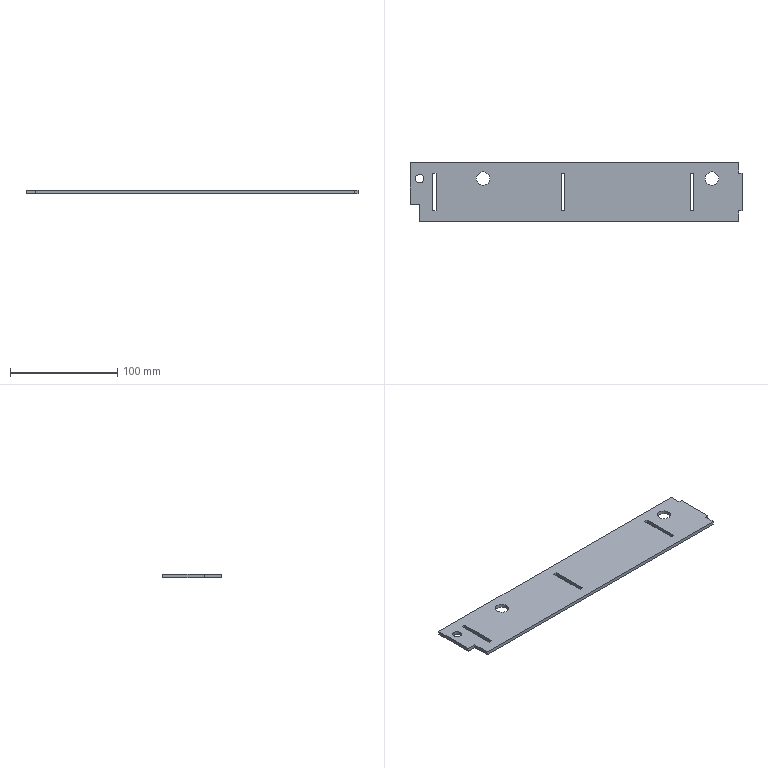Part | SolidWorks | features FlatPattern 1, SMBaseFlange 1, SheetMetal 1 | 1 solid | 30 faces | box 309 x 55 x 3.2 mm | volume 51735 mm3 | plane 24 | cylinder 6 | commonest cylinder face diameters 12.5 x4 8 x2
STEP:
#1=CARTESIAN_POINT('',(186.75,-15.,3.2));
#2=VERTEX_POINT('',#1);
#3=CARTESIAN_POINT('',(199.25,-15.,3.2));
#4=VERTEX_POINT('',#3);
#5=CARTESIAN_POINT('',(193.,-15.,3.2));
#6=DIRECTION('',(0.,0.,1.));
#7=DIRECTION('',(1.,0.,0.));
#8=AXIS2_PLACEMENT_3D('',#5,#6,#7);
#9=CIRCLE('',#8,6.25);
#10=EDGE_CURVE('',#2,#4,#9,.T.);
#11=ORIENTED_EDGE('',*,*,#10,.T.);
#12=CARTESIAN_POINT('',(199.25,-15.,0.));
#13=VERTEX_POINT('',#12);
#14=CARTESIAN_POINT('',(199.25,-15.,3.2));
#15=DIRECTION('',(0.,0.,-1.));
#16=VECTOR('',#15,1000.);
#17=LINE('',#14,#16);
#18=EDGE_CURVE('',#4,#13,#17,.T.);
#19=ORIENTED_EDGE('',*,*,#18,.T.);
#20=CARTESIAN_POINT('',(186.75,-15.,0.));
#21=VERTEX_POINT('',#20);
#22=CARTESIAN_POINT('',(193.,-15.,0.));
#23=DIRECTION('',(0.,0.,1.));
#24=DIRECTION('',(1.,0.,0.));
#25=AXIS2_PLACEMENT_3D('',#22,#23,#24);
#26=CIRCLE('',#25,6.25);
#27=EDGE_CURVE('',#21,#13,#26,.T.);
#28=ORIENTED_EDGE('',*,*,#27,.F.);
#29=CARTESIAN_POINT('',(186.75,-15.,3.2));
#30=DIRECTION('',(0.,0.,-1.));
#31=VECTOR('',#30,1000.);
#32=LINE('',#29,#31);
#33=EDGE_CURVE('',#2,#21,#32,.T.);
#34=ORIENTED_EDGE('',*,*,#33,.F.);
#35=EDGE_LOOP('',(#11,#19,#28,#34));
#36=FACE_OUTER_BOUND('',#35,.T.);
#37=CARTESIAN_POINT('',(193.,-15.,3.2));
#38=DIRECTION('',(0.,0.,-1.));
#39=DIRECTION('',(-1.,0.,0.));
#40=AXIS2_PLACEMENT_3D('',#37,#38,#39);
#41=CYLINDRICAL_SURFACE('',#40,6.25);
#42=ADVANCED_FACE('',(#36),#41,.F.);
#43=CARTESIAN_POINT('',(-26.25,-15.,3.2));
#44=VERTEX_POINT('',#43);
#45=CARTESIAN_POINT('',(-13.75,-15.,3.2));
#46=VERTEX_POINT('',#45);
#47=CARTESIAN_POINT('',(-20.,-15.,3.2));
#48=DIRECTION('',(0.,0.,1.));
#49=DIRECTION('',(1.,0.,0.));
#50=AXIS2_PLACEMENT_3D('',#47,#48,#49);
#51=CIRCLE('',#50,6.25);
#52=EDGE_CURVE('',#44,#46,#51,.T.);
#53=ORIENTED_EDGE('',*,*,#52,.T.);
#54=CARTESIAN_POINT('',(-13.75,-15.,0.));
#55=VERTEX_POINT('',#54);
#56=CARTESIAN_POINT('',(-13.75,-15.,3.2));
#57=DIRECTION('',(0.,0.,-1.));
#58=VECTOR('',#57,1000.);
#59=LINE('',#56,#58);
#60=EDGE_CURVE('',#46,#55,#59,.T.);
#61=ORIENTED_EDGE('',*,*,#60,.T.);
#62=CARTESIAN_POINT('',(-26.25,-15.,0.));
#63=VERTEX_POINT('',#62);
#64=CARTESIAN_POINT('',(-20.,-15.,0.));
#65=DIRECTION('',(0.,0.,1.));
#66=DIRECTION('',(1.,0.,0.));
#67=AXIS2_PLACEMENT_3D('',#64,#65,#66);
#68=CIRCLE('',#67,6.25);
#69=EDGE_CURVE('',#63,#55,#68,.T.);
#70=ORIENTED_EDGE('',*,*,#69,.F.);
#71=CARTESIAN_POINT('',(-26.25,-15.,3.2));
#72=DIRECTION('',(0.,0.,-1.));
#73=VECTOR('',#72,1000.);
#74=LINE('',#71,#73);
#75=EDGE_CURVE('',#44,#63,#74,.T.);
#76=ORIENTED_EDGE('',*,*,#75,.F.);
#77=EDGE_LOOP('',(#53,#61,#70,#76));
#78=FACE_OUTER_BOUND('',#77,.T.);
#79=CARTESIAN_POINT('',(-20.,-15.,3.2));
#80=DIRECTION('',(0.,0.,-1.));
#81=DIRECTION('',(-1.,0.,0.));
#82=AXIS2_PLACEMENT_3D('',#79,#80,#81);
#83=CYLINDRICAL_SURFACE('',#82,6.25);
#84=ADVANCED_FACE('',(#78),#83,.F.);
#85=CARTESIAN_POINT('',(-83.,-15.,3.2));
#86=VERTEX_POINT('',#85);
#87=CARTESIAN_POINT('',(-75.,-15.,3.2));
#88=VERTEX_POINT('',#87);
#89=CARTESIAN_POINT('',(-79.,-15.,3.2));
#90=DIRECTION('',(0.,0.,1.));
#91=DIRECTION('',(1.,0.,0.));
#92=AXIS2_PLACEMENT_3D('',#89,#90,#91);
#93=CIRCLE('',#92,4.);
#94=EDGE_CURVE('',#86,#88,#93,.T.);
#95=ORIENTED_EDGE('',*,*,#94,.T.);
#96=CARTESIAN_POINT('',(-75.,-15.,0.));
#97=VERTEX_POINT('',#96);
#98=CARTESIAN_POINT('',(-75.,-15.,3.2));
#99=DIRECTION('',(0.,0.,-1.));
#100=VECTOR('',#99,1000.);
#101=LINE('',#98,#100);
#102=EDGE_CURVE('',#88,#97,#101,.T.);
#103=ORIENTED_EDGE('',*,*,#102,.T.);
#104=CARTESIAN_POINT('',(-83.,-15.,0.));
#105=VERTEX_POINT('',#104);
#106=CARTESIAN_POINT('',(-79.,-15.,0.));
#107=DIRECTION('',(0.,0.,1.));
#108=DIRECTION('',(1.,0.,0.));
#109=AXIS2_PLACEMENT_3D('',#106,#107,#108);
#110=CIRCLE('',#109,4.);
#111=EDGE_CURVE('',#105,#97,#110,.T.);
#112=ORIENTED_EDGE('',*,*,#111,.F.);
#113=CARTESIAN_POINT('',(-83.,-15.,3.2));
#114=DIRECTION('',(0.,0.,-1.));
#115=VECTOR('',#114,1000.);
#116=LINE('',#113,#115);
#117=EDGE_CURVE('',#86,#105,#116,.T.);
#118=ORIENTED_EDGE('',*,*,#117,.F.);
#119=EDGE_LOOP('',(#95,#103,#112,#118));
#120=FACE_OUTER_BOUND('',#119,.T.);
#121=CARTESIAN_POINT('',(-79.,-15.,3.2));
#122=DIRECTION('',(0.,0.,-1.));
#123=DIRECTION('',(-1.,0.,0.));
#124=AXIS2_PLACEMENT_3D('',#121,#122,#123);
#125=CYLINDRICAL_SURFACE('',#124,4.);
#126=ADVANCED_FACE('',(#120),#125,.F.);
#127=ORIENTED_EDGE('',*,*,#52,.F.);
#128=CARTESIAN_POINT('',(-20.,-15.,3.2));
#129=DIRECTION('',(0.,0.,1.));
#130=DIRECTION('',(1.,0.,0.));
#131=AXIS2_PLACEMENT_3D('',#128,#129,#130);
#132=CIRCLE('',#131,6.25);
#133=EDGE_CURVE('',#46,#44,#132,.T.);
#134=ORIENTED_EDGE('',*,*,#133,.F.);
#135=EDGE_LOOP('',(#127,#134));
#136=FACE_BOUND('',#135,.T.);
#137=CARTESIAN_POINT('',(-67.,-45.,3.2));
#138=VERTEX_POINT('',#137);
#139=CARTESIAN_POINT('',(-63.8,-45.,3.2));
#140=VERTEX_POINT('',#139);
#141=CARTESIAN_POINT('',(-67.,-45.,3.2));
#142=DIRECTION('',(1.,0.,0.));
#143=VECTOR('',#142,1000.);
#144=LINE('',#141,#143);
#145=EDGE_CURVE('',#138,#140,#144,.T.);
#146=ORIENTED_EDGE('',*,*,#145,.F.);
#147=CARTESIAN_POINT('',(-67.,-10.,3.2));
#148=VERTEX_POINT('',#147);
#149=CARTESIAN_POINT('',(-67.,-45.,3.2));
#150=DIRECTION('',(0.,-1.,0.));
#151=VECTOR('',#150,1000.);
#152=LINE('',#149,#151);
#153=EDGE_CURVE('',#148,#138,#152,.T.);
#154=ORIENTED_EDGE('',*,*,#153,.F.);
#155=CARTESIAN_POINT('',(-63.8,-10.,3.2));
#156=VERTEX_POINT('',#155);
#157=CARTESIAN_POINT('',(-67.,-10.,3.2));
#158=DIRECTION('',(-1.,0.,0.));
#159=VECTOR('',#158,1000.);
#160=LINE('',#157,#159);
#161=EDGE_CURVE('',#156,#148,#160,.T.);
#162=ORIENTED_EDGE('',*,*,#161,.F.);
#163=CARTESIAN_POINT('',(-63.8,-45.,3.2));
#164=DIRECTION('',(0.,1.,0.));
#165=VECTOR('',#164,1000.);
#166=LINE('',#163,#165);
#167=EDGE_CURVE('',#140,#156,#166,.T.);
#168=ORIENTED_EDGE('',*,*,#167,.F.);
#169=EDGE_LOOP('',(#146,#154,#162,#168));
#170=FACE_BOUND('',#169,.T.);
#171=CARTESIAN_POINT('',(-88.,-39.,3.2));
#172=VERTEX_POINT('',#171);
#173=CARTESIAN_POINT('',(-79.5,-39.,3.2));
#174=VERTEX_POINT('',#173);
#175=CARTESIAN_POINT('',(-88.,-39.,3.2));
#176=DIRECTION('',(1.,0.,0.));
#177=VECTOR('',#176,1000.);
#178=LINE('',#175,#177);
#179=EDGE_CURVE('',#172,#174,#178,.T.);
#180=ORIENTED_EDGE('',*,*,#179,.T.);
#181=CARTESIAN_POINT('',(-79.5,-55.,3.2));
#182=VERTEX_POINT('',#181);
#183=CARTESIAN_POINT('',(-79.5,-55.,3.2));
#184=DIRECTION('',(0.,-1.,0.));
#185=VECTOR('',#184,1000.);
#186=LINE('',#183,#185);
#187=EDGE_CURVE('',#174,#182,#186,.T.);
#188=ORIENTED_EDGE('',*,*,#187,.T.);
#189=CARTESIAN_POINT('',(218.,-55.,3.2));
#190=VERTEX_POINT('',#189);
#191=CARTESIAN_POINT('',(218.,-55.,3.2));
#192=DIRECTION('',(1.,0.,0.));
#193=VECTOR('',#192,1000.);
#194=LINE('',#191,#193);
#195=EDGE_CURVE('',#182,#190,#194,.T.);
#196=ORIENTED_EDGE('',*,*,#195,.T.);
#197=CARTESIAN_POINT('',(218.,-45.,3.2));
#198=VERTEX_POINT('',#197);
#199=CARTESIAN_POINT('',(218.,-45.,3.2));
#200=DIRECTION('',(0.,1.,0.));
#201=VECTOR('',#200,1000.);
#202=LINE('',#199,#201);
#203=EDGE_CURVE('',#190,#198,#202,.T.);
#204=ORIENTED_EDGE('',*,*,#203,.T.);
#205=CARTESIAN_POINT('',(221.,-45.,3.2));
#206=VERTEX_POINT('',#205);
#207=CARTESIAN_POINT('',(221.,-45.,3.2));
#208=DIRECTION('',(1.,0.,0.));
#209=VECTOR('',#208,1000.);
#210=LINE('',#207,#209);
#211=EDGE_CURVE('',#198,#206,#210,.T.);
#212=ORIENTED_EDGE('',*,*,#211,.T.);
#213=CARTESIAN_POINT('',(221.,-10.,3.2));
#214=VERTEX_POINT('',#213);
#215=CARTESIAN_POINT('',(221.,-10.,3.2));
#216=DIRECTION('',(0.,1.,0.));
#217=VECTOR('',#216,1000.);
#218=LINE('',#215,#217);
#219=EDGE_CURVE('',#206,#214,#218,.T.);
#220=ORIENTED_EDGE('',*,*,#219,.T.);
#221=CARTESIAN_POINT('',(218.,-10.,3.2));
#222=VERTEX_POINT('',#221);
#223=CARTESIAN_POINT('',(218.,-10.,3.2));
#224=DIRECTION('',(-1.,0.,0.));
#225=VECTOR('',#224,1000.);
#226=LINE('',#223,#225);
#227=EDGE_CURVE('',#214,#222,#226,.T.);
#228=ORIENTED_EDGE('',*,*,#227,.T.);
#229=CARTESIAN_POINT('',(218.,0.,3.2));
#230=VERTEX_POINT('',#229);
#231=CARTESIAN_POINT('',(218.,0.,3.2));
#232=DIRECTION('',(0.,1.,0.));
#233=VECTOR('',#232,1000.);
#234=LINE('',#231,#233);
#235=EDGE_CURVE('',#222,#230,#234,.T.);
#236=ORIENTED_EDGE('',*,*,#235,.T.);
#237=CARTESIAN_POINT('',(-88.,0.,3.2));
#238=VERTEX_POINT('',#237);
#239=CARTESIAN_POINT('',(-88.,0.,3.2));
#240=DIRECTION('',(-1.,0.,0.));
#241=VECTOR('',#240,1000.);
#242=LINE('',#239,#241);
#243=EDGE_CURVE('',#230,#238,#242,.T.);
#244=ORIENTED_EDGE('',*,*,#243,.T.);
#245=CARTESIAN_POINT('',(-88.,0.,3.2));
#246=DIRECTION('',(0.,-1.,0.));
#247=VECTOR('',#246,1000.);
#248=LINE('',#245,#247);
#249=EDGE_CURVE('',#238,#172,#248,.T.);
#250=ORIENTED_EDGE('',*,*,#249,.T.);
#251=EDGE_LOOP('',(#180,#188,#196,#204,#212,#220,#228,#236,#244,#250));
#252=FACE_OUTER_BOUND('',#251,.T.);
#253=ORIENTED_EDGE('',*,*,#94,.F.);
#254=CARTESIAN_POINT('',(-79.,-15.,3.2));
#255=DIRECTION('',(0.,0.,1.));
#256=DIRECTION('',(1.,0.,0.));
#257=AXIS2_PLACEMENT_3D('',#254,#255,#256);
#258=CIRCLE('',#257,4.);
#259=EDGE_CURVE('',#88,#86,#258,.T.);
#260=ORIENTED_EDGE('',*,*,#259,.F.);
#261=EDGE_LOOP('',(#253,#260));
#262=FACE_BOUND('',#261,.T.);
#263=ORIENTED_EDGE('',*,*,#10,.F.);
#264=CARTESIAN_POINT('',(193.,-15.,3.2));
#265=DIRECTION('',(0.,0.,1.));
#266=DIRECTION('',(1.,0.,0.));
#267=AXIS2_PLACEMENT_3D('',#264,#265,#266);
#268=CIRCLE('',#267,6.25);
#269=EDGE_CURVE('',#4,#2,#268,.T.);
#270=ORIENTED_EDGE('',*,*,#269,.F.);
#271=EDGE_LOOP('',(#263,#270));
#272=FACE_BOUND('',#271,.T.);
#273=CARTESIAN_POINT('',(53.,-45.,3.2));
#274=VERTEX_POINT('',#273);
#275=CARTESIAN_POINT('',(56.2,-45.,3.2));
#276=VERTEX_POINT('',#275);
#277=CARTESIAN_POINT('',(53.,-45.,3.2));
#278=DIRECTION('',(1.,0.,0.));
#279=VECTOR('',#278,1000.);
#280=LINE('',#277,#279);
#281=EDGE_CURVE('',#274,#276,#280,.T.);
#282=ORIENTED_EDGE('',*,*,#281,.F.);
#283=CARTESIAN_POINT('',(53.,-10.,3.2));
#284=VERTEX_POINT('',#283);
#285=CARTESIAN_POINT('',(53.,-45.,3.2));
#286=DIRECTION('',(0.,-1.,0.));
#287=VECTOR('',#286,1000.);
#288=LINE('',#285,#287);
#289=EDGE_CURVE('',#284,#274,#288,.T.);
#290=ORIENTED_EDGE('',*,*,#289,.F.);
#291=CARTESIAN_POINT('',(56.2,-10.,3.2));
#292=VERTEX_POINT('',#291);
#293=CARTESIAN_POINT('',(53.,-10.,3.2));
#294=DIRECTION('',(-1.,0.,0.));
#295=VECTOR('',#294,1000.);
#296=LINE('',#293,#295);
#297=EDGE_CURVE('',#292,#284,#296,.T.);
#298=ORIENTED_EDGE('',*,*,#297,.F.);
#299=CARTESIAN_POINT('',(56.2,-45.,3.2));
#300=DIRECTION('',(0.,1.,0.));
#301=VECTOR('',#300,1000.);
#302=LINE('',#299,#301);
#303=EDGE_CURVE('',#276,#292,#302,.T.);
#304=ORIENTED_EDGE('',*,*,#303,.F.);
#305=EDGE_LOOP('',(#282,#290,#298,#304));
#306=FACE_BOUND('',#305,.T.);
#307=CARTESIAN_POINT('',(173.,-45.,3.2));
#308=VERTEX_POINT('',#307);
#309=CARTESIAN_POINT('',(176.2,-45.,3.2));
#310=VERTEX_POINT('',#309);
#311=CARTESIAN_POINT('',(173.,-45.,3.2));
#312=DIRECTION('',(1.,0.,0.));
#313=VECTOR('',#312,1000.);
#314=LINE('',#311,#313);
#315=EDGE_CURVE('',#308,#310,#314,.T.);
#316=ORIENTED_EDGE('',*,*,#315,.F.);
#317=CARTESIAN_POINT('',(173.,-10.,3.2));
#318=VERTEX_POINT('',#317);
#319=CARTESIAN_POINT('',(173.,-45.,3.2));
#320=DIRECTION('',(0.,-1.,0.));
#321=VECTOR('',#320,1000.);
#322=LINE('',#319,#321);
#323=EDGE_CURVE('',#318,#308,#322,.T.);
#324=ORIENTED_EDGE('',*,*,#323,.F.);
#325=CARTESIAN_POINT('',(176.2,-10.,3.2));
#326=VERTEX_POINT('',#325);
#327=CARTESIAN_POINT('',(173.,-10.,3.2));
#328=DIRECTION('',(-1.,0.,0.));
#329=VECTOR('',#328,1000.);
#330=LINE('',#327,#329);
#331=EDGE_CURVE('',#326,#318,#330,.T.);
#332=ORIENTED_EDGE('',*,*,#331,.F.);
#333=CARTESIAN_POINT('',(176.2,-45.,3.2));
#334=DIRECTION('',(0.,1.,0.));
#335=VECTOR('',#334,1000.);
#336=LINE('',#333,#335);
#337=EDGE_CURVE('',#310,#326,#336,.T.);
#338=ORIENTED_EDGE('',*,*,#337,.F.);
#339=EDGE_LOOP('',(#316,#324,#332,#338));
#340=FACE_BOUND('',#339,.T.);
#341=CARTESIAN_POINT('',(0.,0.,3.2));
#342=DIRECTION('',(0.,0.,1.));
#343=DIRECTION('',(1.,0.,0.));
#344=AXIS2_PLACEMENT_3D('',#341,#342,#343);
#345=PLANE('',#344);
#346=ADVANCED_FACE('',(#136,#170,#252,#262,#272,#306,#340),#345,.T.);
#347=CARTESIAN_POINT('',(53.,-10.,0.));
#348=VERTEX_POINT('',#347);
#349=CARTESIAN_POINT('',(53.,-45.,0.));
#350=VERTEX_POINT('',#349);
#351=CARTESIAN_POINT('',(53.,-45.,0.));
#352=DIRECTION('',(0.,-1.,0.));
#353=VECTOR('',#352,1000.);
#354=LINE('',#351,#353);
#355=EDGE_CURVE('',#348,#350,#354,.T.);
#356=ORIENTED_EDGE('',*,*,#355,.T.);
#357=CARTESIAN_POINT('',(56.2,-45.,0.));
#358=VERTEX_POINT('',#357);
#359=CARTESIAN_POINT('',(53.,-45.,0.));
#360=DIRECTION('',(1.,0.,0.));
#361=VECTOR('',#360,1000.);
#362=LINE('',#359,#361);
#363=EDGE_CURVE('',#350,#358,#362,.T.);
#364=ORIENTED_EDGE('',*,*,#363,.T.);
#365=CARTESIAN_POINT('',(56.2,-10.,0.));
#366=VERTEX_POINT('',#365);
#367=CARTESIAN_POINT('',(56.2,-45.,0.));
#368=DIRECTION('',(0.,1.,0.));
#369=VECTOR('',#368,1000.);
#370=LINE('',#367,#369);
#371=EDGE_CURVE('',#358,#366,#370,.T.);
#372=ORIENTED_EDGE('',*,*,#371,.T.);
#373=CARTESIAN_POINT('',(53.,-10.,0.));
#374=DIRECTION('',(-1.,0.,0.));
#375=VECTOR('',#374,1000.);
#376=LINE('',#373,#375);
#377=EDGE_CURVE('',#366,#348,#376,.T.);
#378=ORIENTED_EDGE('',*,*,#377,.T.);
#379=EDGE_LOOP('',(#356,#364,#372,#378));
#380=FACE_BOUND('',#379,.T.);
#381=CARTESIAN_POINT('',(-88.,-39.,0.));
#382=VERTEX_POINT('',#381);
#383=CARTESIAN_POINT('',(-79.5,-39.,0.));
#384=VERTEX_POINT('',#383);
#385=CARTESIAN_POINT('',(-88.,-39.,0.));
#386=DIRECTION('',(1.,0.,0.));
#387=VECTOR('',#386,1000.);
#388=LINE('',#385,#387);
#389=EDGE_CURVE('',#382,#384,#388,.T.);
#390=ORIENTED_EDGE('',*,*,#389,.F.);
#391=CARTESIAN_POINT('',(-88.,0.,0.));
#392=VERTEX_POINT('',#391);
#393=CARTESIAN_POINT('',(-88.,0.,0.));
#394=DIRECTION('',(0.,-1.,0.));
#395=VECTOR('',#394,1000.);
#396=LINE('',#393,#395);
#397=EDGE_CURVE('',#392,#382,#396,.T.);
#398=ORIENTED_EDGE('',*,*,#397,.F.);
#399=CARTESIAN_POINT('',(218.,0.,0.));
#400=VERTEX_POINT('',#399);
#401=CARTESIAN_POINT('',(-88.,0.,0.));
#402=DIRECTION('',(-1.,0.,0.));
#403=VECTOR('',#402,1000.);
#404=LINE('',#401,#403);
#405=EDGE_CURVE('',#400,#392,#404,.T.);
#406=ORIENTED_EDGE('',*,*,#405,.F.);
#407=CARTESIAN_POINT('',(218.,-10.,0.));
#408=VERTEX_POINT('',#407);
#409=CARTESIAN_POINT('',(218.,0.,0.));
#410=DIRECTION('',(0.,1.,0.));
#411=VECTOR('',#410,1000.);
#412=LINE('',#409,#411);
#413=EDGE_CURVE('',#408,#400,#412,.T.);
#414=ORIENTED_EDGE('',*,*,#413,.F.);
#415=CARTESIAN_POINT('',(221.,-10.,0.));
#416=VERTEX_POINT('',#415);
#417=CARTESIAN_POINT('',(218.,-10.,0.));
#418=DIRECTION('',(-1.,0.,0.));
#419=VECTOR('',#418,1000.);
#420=LINE('',#417,#419);
#421=EDGE_CURVE('',#416,#408,#420,.T.);
#422=ORIENTED_EDGE('',*,*,#421,.F.);
#423=CARTESIAN_POINT('',(221.,-45.,0.));
#424=VERTEX_POINT('',#423);
#425=CARTESIAN_POINT('',(221.,-10.,0.));
#426=DIRECTION('',(0.,1.,0.));
#427=VECTOR('',#426,1000.);
#428=LINE('',#425,#427);
#429=EDGE_CURVE('',#424,#416,#428,.T.);
#430=ORIENTED_EDGE('',*,*,#429,.F.);
#431=CARTESIAN_POINT('',(218.,-45.,0.));
#432=VERTEX_POINT('',#431);
#433=CARTESIAN_POINT('',(221.,-45.,0.));
#434=DIRECTION('',(1.,0.,0.));
#435=VECTOR('',#434,1000.);
#436=LINE('',#433,#435);
#437=EDGE_CURVE('',#432,#424,#436,.T.);
#438=ORIENTED_EDGE('',*,*,#437,.F.);
#439=CARTESIAN_POINT('',(218.,-55.,0.));
#440=VERTEX_POINT('',#439);
#441=CARTESIAN_POINT('',(218.,-45.,0.));
#442=DIRECTION('',(0.,1.,0.));
#443=VECTOR('',#442,1000.);
#444=LINE('',#441,#443);
#445=EDGE_CURVE('',#440,#432,#444,.T.);
#446=ORIENTED_EDGE('',*,*,#445,.F.);
#447=CARTESIAN_POINT('',(-79.5,-55.,0.));
#448=VERTEX_POINT('',#447);
#449=CARTESIAN_POINT('',(218.,-55.,0.));
#450=DIRECTION('',(1.,0.,0.));
#451=VECTOR('',#450,1000.);
#452=LINE('',#449,#451);
#453=EDGE_CURVE('',#448,#440,#452,.T.);
#454=ORIENTED_EDGE('',*,*,#453,.F.);
#455=CARTESIAN_POINT('',(-79.5,-55.,0.));
#456=DIRECTION('',(0.,-1.,0.));
#457=VECTOR('',#456,1000.);
#458=LINE('',#455,#457);
#459=EDGE_CURVE('',#384,#448,#458,.T.);
#460=ORIENTED_EDGE('',*,*,#459,.F.);
#461=EDGE_LOOP('',(#390,#398,#406,#414,#422,#430,#438,#446,#454,#460));
#462=FACE_OUTER_BOUND('',#461,.T.);
#463=CARTESIAN_POINT('',(-67.,-10.,0.));
#464=VERTEX_POINT('',#463);
#465=CARTESIAN_POINT('',(-67.,-45.,0.));
#466=VERTEX_POINT('',#465);
#467=CARTESIAN_POINT('',(-67.,-45.,0.));
#468=DIRECTION('',(0.,-1.,0.));
#469=VECTOR('',#468,1000.);
#470=LINE('',#467,#469);
#471=EDGE_CURVE('',#464,#466,#470,.T.);
#472=ORIENTED_EDGE('',*,*,#471,.T.);
#473=CARTESIAN_POINT('',(-63.8,-45.,0.));
#474=VERTEX_POINT('',#473);
#475=CARTESIAN_POINT('',(-67.,-45.,0.));
#476=DIRECTION('',(1.,0.,0.));
#477=VECTOR('',#476,1000.);
#478=LINE('',#475,#477);
#479=EDGE_CURVE('',#466,#474,#478,.T.);
#480=ORIENTED_EDGE('',*,*,#479,.T.);
#481=CARTESIAN_POINT('',(-63.8,-10.,0.));
#482=VERTEX_POINT('',#481);
#483=CARTESIAN_POINT('',(-63.8,-45.,0.));
#484=DIRECTION('',(0.,1.,0.));
#485=VECTOR('',#484,1000.);
#486=LINE('',#483,#485);
#487=EDGE_CURVE('',#474,#482,#486,.T.);
#488=ORIENTED_EDGE('',*,*,#487,.T.);
#489=CARTESIAN_POINT('',(-67.,-10.,0.));
#490=DIRECTION('',(-1.,0.,0.));
#491=VECTOR('',#490,1000.);
#492=LINE('',#489,#491);
#493=EDGE_CURVE('',#482,#464,#492,.T.);
#494=ORIENTED_EDGE('',*,*,#493,.T.);
#495=EDGE_LOOP('',(#472,#480,#488,#494));
#496=FACE_BOUND('',#495,.T.);
#497=ORIENTED_EDGE('',*,*,#111,.T.);
#498=CARTESIAN_POINT('',(-79.,-15.,0.));
#499=DIRECTION('',(0.,0.,1.));
#500=DIRECTION('',(1.,0.,0.));
#501=AXIS2_PLACEMENT_3D('',#498,#499,#500);
#502=CIRCLE('',#501,4.);
#503=EDGE_CURVE('',#97,#105,#502,.T.);
#504=ORIENTED_EDGE('',*,*,#503,.T.);
#505=EDGE_LOOP('',(#497,#504));
#506=FACE_BOUND('',#505,.T.);
#507=ORIENTED_EDGE('',*,*,#69,.T.);
#508=CARTESIAN_POINT('',(-20.,-15.,0.));
#509=DIRECTION('',(0.,0.,1.));
#510=DIRECTION('',(1.,0.,0.));
#511=AXIS2_PLACEMENT_3D('',#508,#509,#510);
#512=CIRCLE('',#511,6.25);
#513=EDGE_CURVE('',#55,#63,#512,.T.);
#514=ORIENTED_EDGE('',*,*,#513,.T.);
#515=EDGE_LOOP('',(#507,#514));
#516=FACE_BOUND('',#515,.T.);
#517=ORIENTED_EDGE('',*,*,#27,.T.);
#518=CARTESIAN_POINT('',(193.,-15.,0.));
#519=DIRECTION('',(0.,0.,1.));
#520=DIRECTION('',(1.,0.,0.));
#521=AXIS2_PLACEMENT_3D('',#518,#519,#520);
#522=CIRCLE('',#521,6.25);
#523=EDGE_CURVE('',#13,#21,#522,.T.);
#524=ORIENTED_EDGE('',*,*,#523,.T.);
#525=EDGE_LOOP('',(#517,#524));
#526=FACE_BOUND('',#525,.T.);
#527=CARTESIAN_POINT('',(173.,-10.,0.));
#528=VERTEX_POINT('',#527);
#529=CARTESIAN_POINT('',(173.,-45.,0.));
#530=VERTEX_POINT('',#529);
#531=CARTESIAN_POINT('',(173.,-45.,0.));
#532=DIRECTION('',(0.,-1.,0.));
#533=VECTOR('',#532,1000.);
#534=LINE('',#531,#533);
#535=EDGE_CURVE('',#528,#530,#534,.T.);
#536=ORIENTED_EDGE('',*,*,#535,.T.);
#537=CARTESIAN_POINT('',(176.2,-45.,0.));
#538=VERTEX_POINT('',#537);
#539=CARTESIAN_POINT('',(173.,-45.,0.));
#540=DIRECTION('',(1.,0.,0.));
#541=VECTOR('',#540,1000.);
#542=LINE('',#539,#541);
#543=EDGE_CURVE('',#530,#538,#542,.T.);
#544=ORIENTED_EDGE('',*,*,#543,.T.);
#545=CARTESIAN_POINT('',(176.2,-10.,0.));
#546=VERTEX_POINT('',#545);
#547=CARTESIAN_POINT('',(176.2,-45.,0.));
#548=DIRECTION('',(0.,1.,0.));
#549=VECTOR('',#548,1000.);
#550=LINE('',#547,#549);
#551=EDGE_CURVE('',#538,#546,#550,.T.);
#552=ORIENTED_EDGE('',*,*,#551,.T.);
#553=CARTESIAN_POINT('',(173.,-10.,0.));
#554=DIRECTION('',(-1.,0.,0.));
#555=VECTOR('',#554,1000.);
#556=LINE('',#553,#555);
#557=EDGE_CURVE('',#546,#528,#556,.T.);
#558=ORIENTED_EDGE('',*,*,#557,.T.);
#559=EDGE_LOOP('',(#536,#544,#552,#558));
#560=FACE_BOUND('',#559,.T.);
#561=CARTESIAN_POINT('',(0.,0.,0.));
#562=DIRECTION('',(0.,0.,1.));
#563=DIRECTION('',(1.,0.,0.));
#564=AXIS2_PLACEMENT_3D('',#561,#562,#563);
#565=PLANE('',#564);
#566=ADVANCED_FACE('',(#380,#462,#496,#506,#516,#526,#560),#565,.F.);
#567=ORIENTED_EDGE('',*,*,#389,.T.);
#568=CARTESIAN_POINT('',(-79.5,-39.,3.2));
#569=DIRECTION('',(0.,0.,-1.));
#570=VECTOR('',#569,1000.);
#571=LINE('',#568,#570);
#572=EDGE_CURVE('',#174,#384,#571,.T.);
#573=ORIENTED_EDGE('',*,*,#572,.F.);
#574=ORIENTED_EDGE('',*,*,#179,.F.);
#575=CARTESIAN_POINT('',(-88.,-39.,3.2));
#576=DIRECTION('',(0.,0.,-1.));
#577=VECTOR('',#576,1000.);
#578=LINE('',#575,#577);
#579=EDGE_CURVE('',#172,#382,#578,.T.);
#580=ORIENTED_EDGE('',*,*,#579,.T.);
#581=EDGE_LOOP('',(#567,#573,#574,#580));
#582=FACE_OUTER_BOUND('',#581,.T.);
#583=CARTESIAN_POINT('',(-88.,-39.,3.2));
#584=DIRECTION('',(0.,1.,0.));
#585=DIRECTION('',(0.,0.,1.));
#586=AXIS2_PLACEMENT_3D('',#583,#584,#585);
#587=PLANE('',#586);
#588=ADVANCED_FACE('',(#582),#587,.F.);
#589=ORIENTED_EDGE('',*,*,#459,.T.);
#590=CARTESIAN_POINT('',(-79.5,-55.,3.2));
#591=DIRECTION('',(0.,0.,-1.));
#592=VECTOR('',#591,1000.);
#593=LINE('',#590,#592);
#594=EDGE_CURVE('',#182,#448,#593,.T.);
#595=ORIENTED_EDGE('',*,*,#594,.F.);
#596=ORIENTED_EDGE('',*,*,#187,.F.);
#597=ORIENTED_EDGE('',*,*,#572,.T.);
#598=EDGE_LOOP('',(#589,#595,#596,#597));
#599=FACE_OUTER_BOUND('',#598,.T.);
#600=CARTESIAN_POINT('',(-79.5,-55.,3.2));
#601=DIRECTION('',(1.,0.,0.));
#602=DIRECTION('',(0.,0.,-1.));
#603=AXIS2_PLACEMENT_3D('',#600,#601,#602);
#604=PLANE('',#603);
#605=ADVANCED_FACE('',(#599),#604,.F.);
#606=ORIENTED_EDGE('',*,*,#453,.T.);
#607=CARTESIAN_POINT('',(218.,-55.,3.2));
#608=DIRECTION('',(0.,0.,-1.));
#609=VECTOR('',#608,1000.);
#610=LINE('',#607,#609);
#611=EDGE_CURVE('',#190,#440,#610,.T.);
#612=ORIENTED_EDGE('',*,*,#611,.F.);
#613=ORIENTED_EDGE('',*,*,#195,.F.);
#614=ORIENTED_EDGE('',*,*,#594,.T.);
#615=EDGE_LOOP('',(#606,#612,#613,#614));
#616=FACE_OUTER_BOUND('',#615,.T.);
#617=CARTESIAN_POINT('',(218.,-55.,3.2));
#618=DIRECTION('',(0.,1.,0.));
#619=DIRECTION('',(-1.,0.,0.));
#620=AXIS2_PLACEMENT_3D('',#617,#618,#619);
#621=PLANE('',#620);
#622=ADVANCED_FACE('',(#616),#621,.F.);
#623=ORIENTED_EDGE('',*,*,#445,.T.);
#624=CARTESIAN_POINT('',(218.,-45.,3.2));
#625=DIRECTION('',(0.,0.,-1.));
#626=VECTOR('',#625,1000.);
#627=LINE('',#624,#626);
#628=EDGE_CURVE('',#198,#432,#627,.T.);
#629=ORIENTED_EDGE('',*,*,#628,.F.);
#630=ORIENTED_EDGE('',*,*,#203,.F.);
#631=ORIENTED_EDGE('',*,*,#611,.T.);
#632=EDGE_LOOP('',(#623,#629,#630,#631));
#633=FACE_OUTER_BOUND('',#632,.T.);
#634=CARTESIAN_POINT('',(218.,-45.,3.2));
#635=DIRECTION('',(-1.,0.,0.));
#636=DIRECTION('',(0.,0.,1.));
#637=AXIS2_PLACEMENT_3D('',#634,#635,#636);
#638=PLANE('',#637);
#639=ADVANCED_FACE('',(#633),#638,.F.);
#640=ORIENTED_EDGE('',*,*,#437,.T.);
#641=CARTESIAN_POINT('',(221.,-45.,3.2));
#642=DIRECTION('',(0.,0.,-1.));
#643=VECTOR('',#642,1000.);
#644=LINE('',#641,#643);
#645=EDGE_CURVE('',#206,#424,#644,.T.);
#646=ORIENTED_EDGE('',*,*,#645,.F.);
#647=ORIENTED_EDGE('',*,*,#211,.F.);
#648=ORIENTED_EDGE('',*,*,#628,.T.);
#649=EDGE_LOOP('',(#640,#646,#647,#648));
#650=FACE_OUTER_BOUND('',#649,.T.);
#651=CARTESIAN_POINT('',(221.,-45.,3.2));
#652=DIRECTION('',(0.,1.,0.));
#653=DIRECTION('',(0.,0.,1.));
#654=AXIS2_PLACEMENT_3D('',#651,#652,#653);
#655=PLANE('',#654);
#656=ADVANCED_FACE('',(#650),#655,.F.);
#657=ORIENTED_EDGE('',*,*,#429,.T.);
#658=CARTESIAN_POINT('',(221.,-10.,3.2));
#659=DIRECTION('',(0.,0.,-1.));
#660=VECTOR('',#659,1000.);
#661=LINE('',#658,#660);
#662=EDGE_CURVE('',#214,#416,#661,.T.);
#663=ORIENTED_EDGE('',*,*,#662,.F.);
#664=ORIENTED_EDGE('',*,*,#219,.F.);
#665=ORIENTED_EDGE('',*,*,#645,.T.);
#666=EDGE_LOOP('',(#657,#663,#664,#665));
#667=FACE_OUTER_BOUND('',#666,.T.);
#668=CARTESIAN_POINT('',(221.,-10.,3.2));
#669=DIRECTION('',(-1.,0.,0.));
#670=DIRECTION('',(0.,0.,1.));
#671=AXIS2_PLACEMENT_3D('',#668,#669,#670);
#672=PLANE('',#671);
#673=ADVANCED_FACE('',(#667),#672,.F.);
#674=ORIENTED_EDGE('',*,*,#421,.T.);
#675=CARTESIAN_POINT('',(218.,-10.,3.2));
#676=DIRECTION('',(0.,0.,-1.));
#677=VECTOR('',#676,1000.);
#678=LINE('',#675,#677);
#679=EDGE_CURVE('',#222,#408,#678,.T.);
#680=ORIENTED_EDGE('',*,*,#679,.F.);
#681=ORIENTED_EDGE('',*,*,#227,.F.);
#682=ORIENTED_EDGE('',*,*,#662,.T.);
#683=EDGE_LOOP('',(#674,#680,#681,#682));
#684=FACE_OUTER_BOUND('',#683,.T.);
#685=CARTESIAN_POINT('',(218.,-10.,3.2));
#686=DIRECTION('',(0.,-1.,0.));
#687=DIRECTION('',(0.,0.,-1.));
#688=AXIS2_PLACEMENT_3D('',#685,#686,#687);
#689=PLANE('',#688);
#690=ADVANCED_FACE('',(#684),#689,.F.);
#691=ORIENTED_EDGE('',*,*,#413,.T.);
#692=CARTESIAN_POINT('',(218.,0.,3.2));
#693=DIRECTION('',(0.,0.,-1.));
#694=VECTOR('',#693,1000.);
#695=LINE('',#692,#694);
#696=EDGE_CURVE('',#230,#400,#695,.T.);
#697=ORIENTED_EDGE('',*,*,#696,.F.);
#698=ORIENTED_EDGE('',*,*,#235,.F.);
#699=ORIENTED_EDGE('',*,*,#679,.T.);
#700=EDGE_LOOP('',(#691,#697,#698,#699));
#701=FACE_OUTER_BOUND('',#700,.T.);
#702=CARTESIAN_POINT('',(218.,0.,3.2));
#703=DIRECTION('',(-1.,0.,0.));
#704=DIRECTION('',(0.,0.,1.));
#705=AXIS2_PLACEMENT_3D('',#702,#703,#704);
#706=PLANE('',#705);
#707=ADVANCED_FACE('',(#701),#706,.F.);
#708=ORIENTED_EDGE('',*,*,#405,.T.);
#709=CARTESIAN_POINT('',(-88.,0.,3.2));
#710=DIRECTION('',(0.,0.,-1.));
#711=VECTOR('',#710,1000.);
#712=LINE('',#709,#711);
#713=EDGE_CURVE('',#238,#392,#712,.T.);
#714=ORIENTED_EDGE('',*,*,#713,.F.);
#715=ORIENTED_EDGE('',*,*,#243,.F.);
#716=ORIENTED_EDGE('',*,*,#696,.T.);
#717=EDGE_LOOP('',(#708,#714,#715,#716));
#718=FACE_OUTER_BOUND('',#717,.T.);
#719=CARTESIAN_POINT('',(-88.,0.,3.2));
#720=DIRECTION('',(0.,-1.,0.));
#721=DIRECTION('',(1.,0.,0.));
#722=AXIS2_PLACEMENT_3D('',#719,#720,#721);
#723=PLANE('',#722);
#724=ADVANCED_FACE('',(#718),#723,.F.);
#725=ORIENTED_EDGE('',*,*,#397,.T.);
#726=ORIENTED_EDGE('',*,*,#579,.F.);
#727=ORIENTED_EDGE('',*,*,#249,.F.);
#728=ORIENTED_EDGE('',*,*,#713,.T.);
#729=EDGE_LOOP('',(#725,#726,#727,#728));
#730=FACE_OUTER_BOUND('',#729,.T.);
#731=CARTESIAN_POINT('',(-88.,0.,3.2));
#732=DIRECTION('',(1.,0.,0.));
#733=DIRECTION('',(0.,1.,0.));
#734=AXIS2_PLACEMENT_3D('',#731,#732,#733);
#735=PLANE('',#734);
#736=ADVANCED_FACE('',(#730),#735,.F.);
#737=ORIENTED_EDGE('',*,*,#471,.F.);
#738=CARTESIAN_POINT('',(-67.,-10.,3.2));
#739=DIRECTION('',(0.,0.,-1.));
#740=VECTOR('',#739,1000.);
#741=LINE('',#738,#740);
#742=EDGE_CURVE('',#148,#464,#741,.T.);
#743=ORIENTED_EDGE('',*,*,#742,.F.);
#744=ORIENTED_EDGE('',*,*,#153,.T.);
#745=CARTESIAN_POINT('',(-67.,-45.,3.2));
#746=DIRECTION('',(0.,0.,-1.));
#747=VECTOR('',#746,1000.);
#748=LINE('',#745,#747);
#749=EDGE_CURVE('',#138,#466,#748,.T.);
#750=ORIENTED_EDGE('',*,*,#749,.T.);
#751=EDGE_LOOP('',(#737,#743,#744,#750));
#752=FACE_OUTER_BOUND('',#751,.T.);
#753=CARTESIAN_POINT('',(-67.,-45.,3.2));
#754=DIRECTION('',(1.,0.,0.));
#755=DIRECTION('',(0.,0.,-1.));
#756=AXIS2_PLACEMENT_3D('',#753,#754,#755);
#757=PLANE('',#756);
#758=ADVANCED_FACE('',(#752),#757,.T.);
#759=ORIENTED_EDGE('',*,*,#479,.F.);
#760=ORIENTED_EDGE('',*,*,#749,.F.);
#761=ORIENTED_EDGE('',*,*,#145,.T.);
#762=CARTESIAN_POINT('',(-63.8,-45.,3.2));
#763=DIRECTION('',(0.,0.,-1.));
#764=VECTOR('',#763,1000.);
#765=LINE('',#762,#764);
#766=EDGE_CURVE('',#140,#474,#765,.T.);
#767=ORIENTED_EDGE('',*,*,#766,.T.);
#768=EDGE_LOOP('',(#759,#760,#761,#767));
#769=FACE_OUTER_BOUND('',#768,.T.);
#770=CARTESIAN_POINT('',(-67.,-45.,3.2));
#771=DIRECTION('',(0.,1.,0.));
#772=DIRECTION('',(0.,0.,1.));
#773=AXIS2_PLACEMENT_3D('',#770,#771,#772);
#774=PLANE('',#773);
#775=ADVANCED_FACE('',(#769),#774,.T.);
#776=ORIENTED_EDGE('',*,*,#487,.F.);
#777=ORIENTED_EDGE('',*,*,#766,.F.);
#778=ORIENTED_EDGE('',*,*,#167,.T.);
#779=CARTESIAN_POINT('',(-63.8,-10.,3.2));
#780=DIRECTION('',(0.,0.,-1.));
#781=VECTOR('',#780,1000.);
#782=LINE('',#779,#781);
#783=EDGE_CURVE('',#156,#482,#782,.T.);
#784=ORIENTED_EDGE('',*,*,#783,.T.);
#785=EDGE_LOOP('',(#776,#777,#778,#784));
#786=FACE_OUTER_BOUND('',#785,.T.);
#787=CARTESIAN_POINT('',(-63.8,-45.,3.2));
#788=DIRECTION('',(-1.,0.,0.));
#789=DIRECTION('',(0.,0.,1.));
#790=AXIS2_PLACEMENT_3D('',#787,#788,#789);
#791=PLANE('',#790);
#792=ADVANCED_FACE('',(#786),#791,.T.);
#793=ORIENTED_EDGE('',*,*,#493,.F.);
#794=ORIENTED_EDGE('',*,*,#783,.F.);
#795=ORIENTED_EDGE('',*,*,#161,.T.);
#796=ORIENTED_EDGE('',*,*,#742,.T.);
#797=EDGE_LOOP('',(#793,#794,#795,#796));
#798=FACE_OUTER_BOUND('',#797,.T.);
#799=CARTESIAN_POINT('',(-67.,-10.,3.2));
#800=DIRECTION('',(0.,-1.,0.));
#801=DIRECTION('',(0.,0.,-1.));
#802=AXIS2_PLACEMENT_3D('',#799,#800,#801);
#803=PLANE('',#802);
#804=ADVANCED_FACE('',(#798),#803,.T.);
#805=ORIENTED_EDGE('',*,*,#102,.F.);
#806=ORIENTED_EDGE('',*,*,#259,.T.);
#807=ORIENTED_EDGE('',*,*,#117,.T.);
#808=ORIENTED_EDGE('',*,*,#503,.F.);
#809=EDGE_LOOP('',(#805,#806,#807,#808));
#810=FACE_OUTER_BOUND('',#809,.T.);
#811=CARTESIAN_POINT('',(-79.,-15.,3.2));
#812=DIRECTION('',(0.,0.,-1.));
#813=DIRECTION('',(-1.,0.,0.));
#814=AXIS2_PLACEMENT_3D('',#811,#812,#813);
#815=CYLINDRICAL_SURFACE('',#814,4.);
#816=ADVANCED_FACE('',(#810),#815,.F.);
#817=ORIENTED_EDGE('',*,*,#60,.F.);
#818=ORIENTED_EDGE('',*,*,#133,.T.);
#819=ORIENTED_EDGE('',*,*,#75,.T.);
#820=ORIENTED_EDGE('',*,*,#513,.F.);
#821=EDGE_LOOP('',(#817,#818,#819,#820));
#822=FACE_OUTER_BOUND('',#821,.T.);
#823=CARTESIAN_POINT('',(-20.,-15.,3.2));
#824=DIRECTION('',(0.,0.,-1.));
#825=DIRECTION('',(-1.,0.,0.));
#826=AXIS2_PLACEMENT_3D('',#823,#824,#825);
#827=CYLINDRICAL_SURFACE('',#826,6.25);
#828=ADVANCED_FACE('',(#822),#827,.F.);
#829=ORIENTED_EDGE('',*,*,#18,.F.);
#830=ORIENTED_EDGE('',*,*,#269,.T.);
#831=ORIENTED_EDGE('',*,*,#33,.T.);
#832=ORIENTED_EDGE('',*,*,#523,.F.);
#833=EDGE_LOOP('',(#829,#830,#831,#832));
#834=FACE_OUTER_BOUND('',#833,.T.);
#835=CARTESIAN_POINT('',(193.,-15.,3.2));
#836=DIRECTION('',(0.,0.,-1.));
#837=DIRECTION('',(-1.,0.,0.));
#838=AXIS2_PLACEMENT_3D('',#835,#836,#837);
#839=CYLINDRICAL_SURFACE('',#838,6.25);
#840=ADVANCED_FACE('',(#834),#839,.F.);
#841=ORIENTED_EDGE('',*,*,#355,.F.);
#842=CARTESIAN_POINT('',(53.,-10.,3.2));
#843=DIRECTION('',(0.,0.,-1.));
#844=VECTOR('',#843,1000.);
#845=LINE('',#842,#844);
#846=EDGE_CURVE('',#284,#348,#845,.T.);
#847=ORIENTED_EDGE('',*,*,#846,.F.);
#848=ORIENTED_EDGE('',*,*,#289,.T.);
#849=CARTESIAN_POINT('',(53.,-45.,3.2));
#850=DIRECTION('',(0.,0.,-1.));
#851=VECTOR('',#850,1000.);
#852=LINE('',#849,#851);
#853=EDGE_CURVE('',#274,#350,#852,.T.);
#854=ORIENTED_EDGE('',*,*,#853,.T.);
#855=EDGE_LOOP('',(#841,#847,#848,#854));
#856=FACE_OUTER_BOUND('',#855,.T.);
#857=CARTESIAN_POINT('',(53.,-45.,3.2));
#858=DIRECTION('',(1.,0.,0.));
#859=DIRECTION('',(0.,0.,-1.));
#860=AXIS2_PLACEMENT_3D('',#857,#858,#859);
#861=PLANE('',#860);
#862=ADVANCED_FACE('',(#856),#861,.T.);
#863=ORIENTED_EDGE('',*,*,#363,.F.);
#864=ORIENTED_EDGE('',*,*,#853,.F.);
#865=ORIENTED_EDGE('',*,*,#281,.T.);
#866=CARTESIAN_POINT('',(56.2,-45.,3.2));
#867=DIRECTION('',(0.,0.,-1.));
#868=VECTOR('',#867,1000.);
#869=LINE('',#866,#868);
#870=EDGE_CURVE('',#276,#358,#869,.T.);
#871=ORIENTED_EDGE('',*,*,#870,.T.);
#872=EDGE_LOOP('',(#863,#864,#865,#871));
#873=FACE_OUTER_BOUND('',#872,.T.);
#874=CARTESIAN_POINT('',(53.,-45.,3.2));
#875=DIRECTION('',(0.,1.,0.));
#876=DIRECTION('',(0.,0.,1.));
#877=AXIS2_PLACEMENT_3D('',#874,#875,#876);
#878=PLANE('',#877);
#879=ADVANCED_FACE('',(#873),#878,.T.);
#880=ORIENTED_EDGE('',*,*,#371,.F.);
#881=ORIENTED_EDGE('',*,*,#870,.F.);
#882=ORIENTED_EDGE('',*,*,#303,.T.);
#883=CARTESIAN_POINT('',(56.2,-10.,3.2));
#884=DIRECTION('',(0.,0.,-1.));
#885=VECTOR('',#884,1000.);
#886=LINE('',#883,#885);
#887=EDGE_CURVE('',#292,#366,#886,.T.);
#888=ORIENTED_EDGE('',*,*,#887,.T.);
#889=EDGE_LOOP('',(#880,#881,#882,#888));
#890=FACE_OUTER_BOUND('',#889,.T.);
#891=CARTESIAN_POINT('',(56.2,-45.,3.2));
#892=DIRECTION('',(-1.,0.,0.));
#893=DIRECTION('',(0.,0.,1.));
#894=AXIS2_PLACEMENT_3D('',#891,#892,#893);
#895=PLANE('',#894);
#896=ADVANCED_FACE('',(#890),#895,.T.);
#897=ORIENTED_EDGE('',*,*,#377,.F.);
#898=ORIENTED_EDGE('',*,*,#887,.F.);
#899=ORIENTED_EDGE('',*,*,#297,.T.);
#900=ORIENTED_EDGE('',*,*,#846,.T.);
#901=EDGE_LOOP('',(#897,#898,#899,#900));
#902=FACE_OUTER_BOUND('',#901,.T.);
#903=CARTESIAN_POINT('',(53.,-10.,3.2));
#904=DIRECTION('',(0.,-1.,0.));
#905=DIRECTION('',(0.,0.,-1.));
#906=AXIS2_PLACEMENT_3D('',#903,#904,#905);
#907=PLANE('',#906);
#908=ADVANCED_FACE('',(#902),#907,.T.);
#909=ORIENTED_EDGE('',*,*,#535,.F.);
#910=CARTESIAN_POINT('',(173.,-10.,3.2));
#911=DIRECTION('',(0.,0.,-1.));
#912=VECTOR('',#911,1000.);
#913=LINE('',#910,#912);
#914=EDGE_CURVE('',#318,#528,#913,.T.);
#915=ORIENTED_EDGE('',*,*,#914,.F.);
#916=ORIENTED_EDGE('',*,*,#323,.T.);
#917=CARTESIAN_POINT('',(173.,-45.,3.2));
#918=DIRECTION('',(0.,0.,-1.));
#919=VECTOR('',#918,1000.);
#920=LINE('',#917,#919);
#921=EDGE_CURVE('',#308,#530,#920,.T.);
#922=ORIENTED_EDGE('',*,*,#921,.T.);
#923=EDGE_LOOP('',(#909,#915,#916,#922));
#924=FACE_OUTER_BOUND('',#923,.T.);
#925=CARTESIAN_POINT('',(173.,-45.,3.2));
#926=DIRECTION('',(1.,0.,0.));
#927=DIRECTION('',(0.,0.,-1.));
#928=AXIS2_PLACEMENT_3D('',#925,#926,#927);
#929=PLANE('',#928);
#930=ADVANCED_FACE('',(#924),#929,.T.);
#931=ORIENTED_EDGE('',*,*,#543,.F.);
#932=ORIENTED_EDGE('',*,*,#921,.F.);
#933=ORIENTED_EDGE('',*,*,#315,.T.);
#934=CARTESIAN_POINT('',(176.2,-45.,3.2));
#935=DIRECTION('',(0.,0.,-1.));
#936=VECTOR('',#935,1000.);
#937=LINE('',#934,#936);
#938=EDGE_CURVE('',#310,#538,#937,.T.);
#939=ORIENTED_EDGE('',*,*,#938,.T.);
#940=EDGE_LOOP('',(#931,#932,#933,#939));
#941=FACE_OUTER_BOUND('',#940,.T.);
#942=CARTESIAN_POINT('',(173.,-45.,3.2));
#943=DIRECTION('',(0.,1.,0.));
#944=DIRECTION('',(0.,0.,1.));
#945=AXIS2_PLACEMENT_3D('',#942,#943,#944);
#946=PLANE('',#945);
#947=ADVANCED_FACE('',(#941),#946,.T.);
#948=ORIENTED_EDGE('',*,*,#551,.F.);
#949=ORIENTED_EDGE('',*,*,#938,.F.);
#950=ORIENTED_EDGE('',*,*,#337,.T.);
#951=CARTESIAN_POINT('',(176.2,-10.,3.2));
#952=DIRECTION('',(0.,0.,-1.));
#953=VECTOR('',#952,1000.);
#954=LINE('',#951,#953);
#955=EDGE_CURVE('',#326,#546,#954,.T.);
#956=ORIENTED_EDGE('',*,*,#955,.T.);
#957=EDGE_LOOP('',(#948,#949,#950,#956));
#958=FACE_OUTER_BOUND('',#957,.T.);
#959=CARTESIAN_POINT('',(176.2,-45.,3.2));
#960=DIRECTION('',(-1.,0.,0.));
#961=DIRECTION('',(0.,0.,1.));
#962=AXIS2_PLACEMENT_3D('',#959,#960,#961);
#963=PLANE('',#962);
#964=ADVANCED_FACE('',(#958),#963,.T.);
#965=ORIENTED_EDGE('',*,*,#557,.F.);
#966=ORIENTED_EDGE('',*,*,#955,.F.);
#967=ORIENTED_EDGE('',*,*,#331,.T.);
#968=ORIENTED_EDGE('',*,*,#914,.T.);
#969=EDGE_LOOP('',(#965,#966,#967,#968));
#970=FACE_OUTER_BOUND('',#969,.T.);
#971=CARTESIAN_POINT('',(173.,-10.,3.2));
#972=DIRECTION('',(0.,-1.,0.));
#973=DIRECTION('',(0.,0.,-1.));
#974=AXIS2_PLACEMENT_3D('',#971,#972,#973);
#975=PLANE('',#974);
#976=ADVANCED_FACE('',(#970),#975,.T.);
#977=CLOSED_SHELL('',(#42,#84,#126,#346,#566,#588,#605,#622,#639,#656,#673,#690,#707,#724,#736,#758,#775,#792,#804,#816,#828,#840,#862,#879,#896,#908,#930,#947,#964,#976));
#978=MANIFOLD_SOLID_BREP('',#977);
#979=CARTESIAN_POINT('',(0.,0.,0.));
#980=DIRECTION('',(0.,0.,1.));
#981=DIRECTION('',(1.,0.,0.));
#982=AXIS2_PLACEMENT_3D('',#979,#980,#981);
#983=(LENGTH_UNIT()NAMED_UNIT(*)SI_UNIT(.MILLI.,.METRE.));
#984=UNCERTAINTY_MEASURE_WITH_UNIT(LENGTH_MEASURE(0.00001),#983,'','');
#985=(NAMED_UNIT(*)PLANE_ANGLE_UNIT()SI_UNIT($,.RADIAN.));
#986=(NAMED_UNIT(*)SI_UNIT($,.STERADIAN.)SOLID_ANGLE_UNIT());
#987=(GEOMETRIC_REPRESENTATION_CONTEXT(3)GLOBAL_UNCERTAINTY_ASSIGNED_CONTEXT((#984))GLOBAL_UNIT_ASSIGNED_CONTEXT((#983,#985,#986))REPRESENTATION_CONTEXT('',''));
#988=ADVANCED_BREP_SHAPE_REPRESENTATION('',(#978,#982),#987);